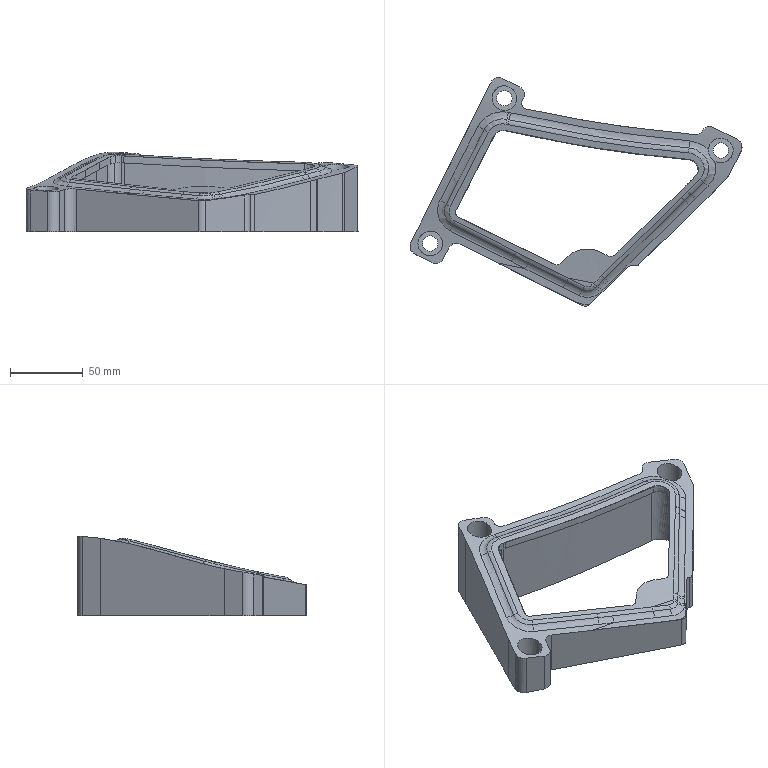Part | STEP file | gslz 2016.10.28-13_id354_x_t | 1 solid | 130 faces | box 228.523 x 157.389 x 54.779 mm | volume 339382 mm3 | spline 63 | other 27 | cylinder 23 | plane 17 | commonest cylinder face diameters 12 x9 8 x3 10.5 x3 17 x3 10 x2 14 x2